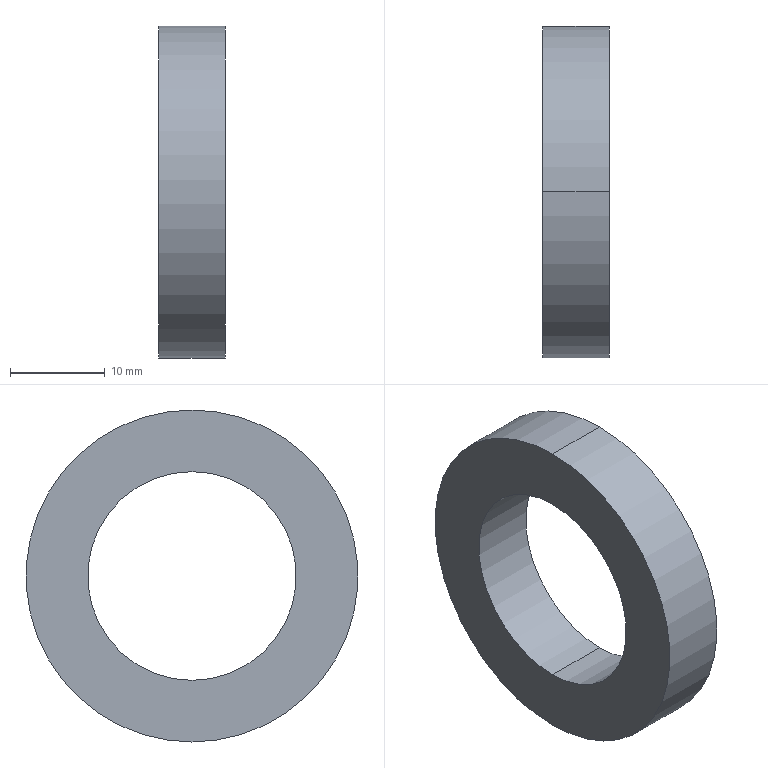Part | SolidWorks | features Extrusion 1 | 1 solid | 6 faces | box 7 x 35 x 35 mm | volume 4074 mm3 | cylinder 4 | plane 2 | commonest cylinder face diameters 22 x2 35 x2
STEP:
#1=CARTESIAN_POINT('',(7.,0.,11.));
#2=VERTEX_POINT('',#1);
#3=CARTESIAN_POINT('',(7.,0.,-11.));
#4=VERTEX_POINT('',#3);
#5=CARTESIAN_POINT('',(7.,0.,0.));
#6=DIRECTION('',(1.,0.,0.));
#7=DIRECTION('',(0.,0.,-1.));
#8=AXIS2_PLACEMENT_3D('',#5,#6,#7);
#9=CIRCLE('',#8,11.);
#10=EDGE_CURVE('',#2,#4,#9,.T.);
#11=ORIENTED_EDGE('',*,*,#10,.T.);
#12=CARTESIAN_POINT('',(0.,0.,-11.));
#13=VERTEX_POINT('',#12);
#14=CARTESIAN_POINT('',(7.,0.,-11.));
#15=DIRECTION('',(-1.,0.,0.));
#16=VECTOR('',#15,1000.);
#17=LINE('',#14,#16);
#18=EDGE_CURVE('',#4,#13,#17,.T.);
#19=ORIENTED_EDGE('',*,*,#18,.T.);
#20=CARTESIAN_POINT('',(0.,0.,11.));
#21=VERTEX_POINT('',#20);
#22=CARTESIAN_POINT('',(0.,0.,0.));
#23=DIRECTION('',(1.,0.,0.));
#24=DIRECTION('',(0.,0.,-1.));
#25=AXIS2_PLACEMENT_3D('',#22,#23,#24);
#26=CIRCLE('',#25,11.);
#27=EDGE_CURVE('',#21,#13,#26,.T.);
#28=ORIENTED_EDGE('',*,*,#27,.F.);
#29=CARTESIAN_POINT('',(7.,0.,11.));
#30=DIRECTION('',(-1.,0.,0.));
#31=VECTOR('',#30,1000.);
#32=LINE('',#29,#31);
#33=EDGE_CURVE('',#2,#21,#32,.T.);
#34=ORIENTED_EDGE('',*,*,#33,.F.);
#35=EDGE_LOOP('',(#11,#19,#28,#34));
#36=FACE_OUTER_BOUND('',#35,.T.);
#37=CARTESIAN_POINT('',(7.,0.,0.));
#38=DIRECTION('',(-1.,0.,0.));
#39=DIRECTION('',(0.,0.,1.));
#40=AXIS2_PLACEMENT_3D('',#37,#38,#39);
#41=CYLINDRICAL_SURFACE('',#40,11.);
#42=ADVANCED_FACE('',(#36),#41,.F.);
#43=CARTESIAN_POINT('',(7.,0.,-17.5));
#44=VERTEX_POINT('',#43);
#45=CARTESIAN_POINT('',(7.,0.,17.5));
#46=VERTEX_POINT('',#45);
#47=CARTESIAN_POINT('',(7.,0.,0.));
#48=DIRECTION('',(1.,0.,0.));
#49=DIRECTION('',(0.,0.,-1.));
#50=AXIS2_PLACEMENT_3D('',#47,#48,#49);
#51=CIRCLE('',#50,17.5);
#52=EDGE_CURVE('',#44,#46,#51,.T.);
#53=ORIENTED_EDGE('',*,*,#52,.F.);
#54=CARTESIAN_POINT('',(0.,0.,-17.5));
#55=VERTEX_POINT('',#54);
#56=CARTESIAN_POINT('',(7.,0.,-17.5));
#57=DIRECTION('',(-1.,0.,0.));
#58=VECTOR('',#57,1000.);
#59=LINE('',#56,#58);
#60=EDGE_CURVE('',#44,#55,#59,.T.);
#61=ORIENTED_EDGE('',*,*,#60,.T.);
#62=CARTESIAN_POINT('',(0.,0.,17.5));
#63=VERTEX_POINT('',#62);
#64=CARTESIAN_POINT('',(0.,0.,0.));
#65=DIRECTION('',(1.,0.,0.));
#66=DIRECTION('',(0.,0.,-1.));
#67=AXIS2_PLACEMENT_3D('',#64,#65,#66);
#68=CIRCLE('',#67,17.5);
#69=EDGE_CURVE('',#55,#63,#68,.T.);
#70=ORIENTED_EDGE('',*,*,#69,.T.);
#71=CARTESIAN_POINT('',(7.,0.,17.5));
#72=DIRECTION('',(-1.,0.,0.));
#73=VECTOR('',#72,1000.);
#74=LINE('',#71,#73);
#75=EDGE_CURVE('',#46,#63,#74,.T.);
#76=ORIENTED_EDGE('',*,*,#75,.F.);
#77=EDGE_LOOP('',(#53,#61,#70,#76));
#78=FACE_OUTER_BOUND('',#77,.T.);
#79=CARTESIAN_POINT('',(7.,0.,0.));
#80=DIRECTION('',(-1.,0.,0.));
#81=DIRECTION('',(0.,0.,1.));
#82=AXIS2_PLACEMENT_3D('',#79,#80,#81);
#83=CYLINDRICAL_SURFACE('',#82,17.5);
#84=ADVANCED_FACE('',(#78),#83,.T.);
#85=CARTESIAN_POINT('',(7.,0.,0.));
#86=DIRECTION('',(1.,0.,0.));
#87=DIRECTION('',(0.,0.,-1.));
#88=AXIS2_PLACEMENT_3D('',#85,#86,#87);
#89=CIRCLE('',#88,17.5);
#90=EDGE_CURVE('',#46,#44,#89,.T.);
#91=ORIENTED_EDGE('',*,*,#90,.T.);
#92=ORIENTED_EDGE('',*,*,#52,.T.);
#93=EDGE_LOOP('',(#91,#92));
#94=FACE_OUTER_BOUND('',#93,.T.);
#95=ORIENTED_EDGE('',*,*,#10,.F.);
#96=CARTESIAN_POINT('',(7.,0.,0.));
#97=DIRECTION('',(1.,0.,0.));
#98=DIRECTION('',(0.,0.,-1.));
#99=AXIS2_PLACEMENT_3D('',#96,#97,#98);
#100=CIRCLE('',#99,11.);
#101=EDGE_CURVE('',#4,#2,#100,.T.);
#102=ORIENTED_EDGE('',*,*,#101,.F.);
#103=EDGE_LOOP('',(#95,#102));
#104=FACE_BOUND('',#103,.T.);
#105=CARTESIAN_POINT('',(7.,0.,0.));
#106=DIRECTION('',(1.,0.,0.));
#107=DIRECTION('',(0.,0.,-1.));
#108=AXIS2_PLACEMENT_3D('',#105,#106,#107);
#109=PLANE('',#108);
#110=ADVANCED_FACE('',(#94,#104),#109,.T.);
#111=CARTESIAN_POINT('',(0.,0.,0.));
#112=DIRECTION('',(1.,0.,0.));
#113=DIRECTION('',(0.,0.,-1.));
#114=AXIS2_PLACEMENT_3D('',#111,#112,#113);
#115=CIRCLE('',#114,17.5);
#116=EDGE_CURVE('',#63,#55,#115,.T.);
#117=ORIENTED_EDGE('',*,*,#116,.F.);
#118=ORIENTED_EDGE('',*,*,#69,.F.);
#119=EDGE_LOOP('',(#117,#118));
#120=FACE_OUTER_BOUND('',#119,.T.);
#121=ORIENTED_EDGE('',*,*,#27,.T.);
#122=CARTESIAN_POINT('',(0.,0.,0.));
#123=DIRECTION('',(1.,0.,0.));
#124=DIRECTION('',(0.,0.,-1.));
#125=AXIS2_PLACEMENT_3D('',#122,#123,#124);
#126=CIRCLE('',#125,11.);
#127=EDGE_CURVE('',#13,#21,#126,.T.);
#128=ORIENTED_EDGE('',*,*,#127,.T.);
#129=EDGE_LOOP('',(#121,#128));
#130=FACE_BOUND('',#129,.T.);
#131=CARTESIAN_POINT('',(0.,0.,0.));
#132=DIRECTION('',(1.,0.,0.));
#133=DIRECTION('',(0.,0.,-1.));
#134=AXIS2_PLACEMENT_3D('',#131,#132,#133);
#135=PLANE('',#134);
#136=ADVANCED_FACE('',(#120,#130),#135,.F.);
#137=ORIENTED_EDGE('',*,*,#60,.F.);
#138=ORIENTED_EDGE('',*,*,#90,.F.);
#139=ORIENTED_EDGE('',*,*,#75,.T.);
#140=ORIENTED_EDGE('',*,*,#116,.T.);
#141=EDGE_LOOP('',(#137,#138,#139,#140));
#142=FACE_OUTER_BOUND('',#141,.T.);
#143=CARTESIAN_POINT('',(7.,0.,0.));
#144=DIRECTION('',(-1.,0.,0.));
#145=DIRECTION('',(0.,0.,1.));
#146=AXIS2_PLACEMENT_3D('',#143,#144,#145);
#147=CYLINDRICAL_SURFACE('',#146,17.5);
#148=ADVANCED_FACE('',(#142),#147,.T.);
#149=ORIENTED_EDGE('',*,*,#18,.F.);
#150=ORIENTED_EDGE('',*,*,#101,.T.);
#151=ORIENTED_EDGE('',*,*,#33,.T.);
#152=ORIENTED_EDGE('',*,*,#127,.F.);
#153=EDGE_LOOP('',(#149,#150,#151,#152));
#154=FACE_OUTER_BOUND('',#153,.T.);
#155=CARTESIAN_POINT('',(7.,0.,0.));
#156=DIRECTION('',(-1.,0.,0.));
#157=DIRECTION('',(0.,0.,1.));
#158=AXIS2_PLACEMENT_3D('',#155,#156,#157);
#159=CYLINDRICAL_SURFACE('',#158,11.);
#160=ADVANCED_FACE('',(#154),#159,.F.);
#161=CLOSED_SHELL('',(#42,#84,#110,#136,#148,#160));
#162=MANIFOLD_SOLID_BREP('',#161);
#163=CARTESIAN_POINT('',(0.,0.,0.));
#164=DIRECTION('',(0.,0.,1.));
#165=DIRECTION('',(1.,0.,0.));
#166=AXIS2_PLACEMENT_3D('',#163,#164,#165);
#167=(LENGTH_UNIT()NAMED_UNIT(*)SI_UNIT(.MILLI.,.METRE.));
#168=UNCERTAINTY_MEASURE_WITH_UNIT(LENGTH_MEASURE(0.00001),#167,'','');
#169=(NAMED_UNIT(*)PLANE_ANGLE_UNIT()SI_UNIT($,.RADIAN.));
#170=(NAMED_UNIT(*)SI_UNIT($,.STERADIAN.)SOLID_ANGLE_UNIT());
#171=(GEOMETRIC_REPRESENTATION_CONTEXT(3)GLOBAL_UNCERTAINTY_ASSIGNED_CONTEXT((#168))GLOBAL_UNIT_ASSIGNED_CONTEXT((#167,#169,#170))REPRESENTATION_CONTEXT('',''));
#172=ADVANCED_BREP_SHAPE_REPRESENTATION('',(#162,#166),#171);